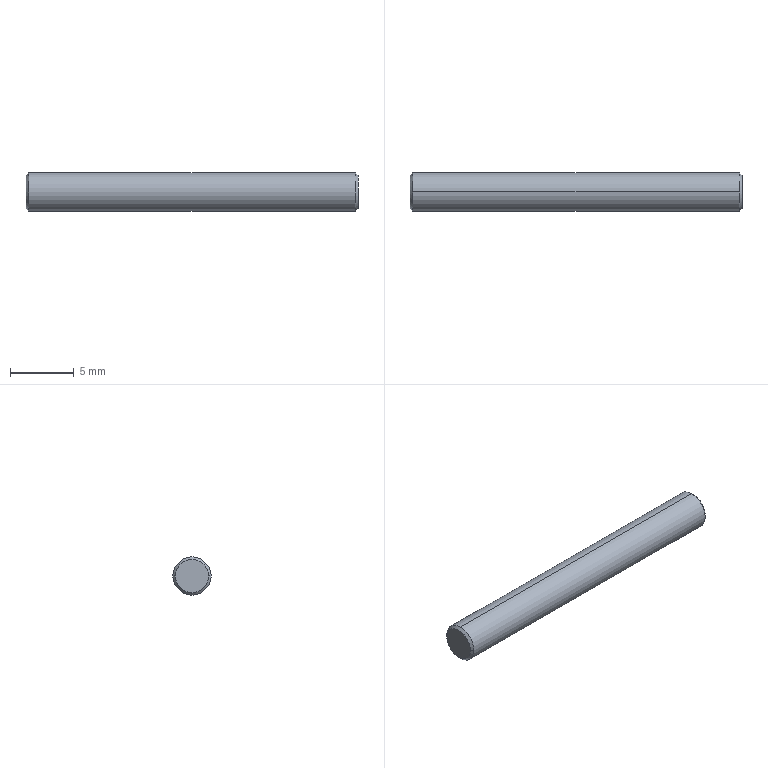Part | STEP file | pin 5_SUS304 | 1 solid | 9 faces | box 26 x 3 x 3 mm | volume 183.423 mm3 | cone 5 | cylinder 2 | plane 2 | commonest cylinder face diameters 3 x2
STEP:
#1=CARTESIAN_POINT('',(0.,0.,0.));
#2=DIRECTION('',(0.,0.,1.));
#3=DIRECTION('',(1.,0.,0.));
#4=AXIS2_PLACEMENT_3D('',#1,#2,#3);
#5=CARTESIAN_POINT('',(12.8,1.5,0.));
#6=VERTEX_POINT('',#5);
#7=CARTESIAN_POINT('',(12.8,0.,-1.5));
#8=VERTEX_POINT('',#7);
#9=CARTESIAN_POINT('',(12.8,0.,0.));
#10=DIRECTION('',(-1.,0.,0.));
#11=DIRECTION('',(0.,0.,1.));
#12=AXIS2_PLACEMENT_3D('',#9,#10,#11);
#13=CIRCLE('',#12,1.5);
#14=CARTESIAN_POINT('',(13.,0.,0.));
#15=DIRECTION('',(-1.,0.,0.));
#16=DIRECTION('',(0.,0.,1.));
#17=AXIS2_PLACEMENT_3D('',#14,#15,#16);
#18=CYLINDRICAL_SURFACE('',#17,1.5);
#19=CARTESIAN_POINT('',(0.,0.2));
#20=DIRECTION('',(1.,0.));
#21=VECTOR('',#20,1.);
#22=LINE('',#19,#21);
#23=(GEOMETRIC_REPRESENTATION_CONTEXT(2)PARAMETRIC_REPRESENTATION_CONTEXT()REPRESENTATION_CONTEXT('',''));
#24=DEFINITIONAL_REPRESENTATION('',(#22),#23);
#25=PCURVE('',#18,#24);
#26=CARTESIAN_POINT('',(12.8,0.,0.));
#27=DIRECTION('',(-1.,0.,0.));
#28=DIRECTION('',(0.,-1.,0.));
#29=AXIS2_PLACEMENT_3D('',#26,#27,#28);
#30=CONICAL_SURFACE('',#29,1.5,0.7854);
#31=CARTESIAN_POINT('',(1.571,0.));
#32=DIRECTION('',(1.,0.));
#33=VECTOR('',#32,1.);
#34=LINE('',#31,#33);
#35=(GEOMETRIC_REPRESENTATION_CONTEXT(2)PARAMETRIC_REPRESENTATION_CONTEXT()REPRESENTATION_CONTEXT('',''));
#36=DEFINITIONAL_REPRESENTATION('',(#34),#35);
#37=PCURVE('',#30,#36);
#38=SURFACE_CURVE('',#13,(#25,#37),.PCURVE_S1.);
#39=EDGE_CURVE('',#6,#8,#38,.T.);
#40=ORIENTED_EDGE('',*,*,#39,.T.);
#41=CARTESIAN_POINT('',(-12.8,0.,-1.5));
#42=VERTEX_POINT('',#41);
#43=CARTESIAN_POINT('',(13.,0.,-1.5));
#44=DIRECTION('',(-1.,0.,0.));
#45=VECTOR('',#44,1.);
#46=LINE('',#43,#45);
#47=CARTESIAN_POINT('',(3.142,0.));
#48=DIRECTION('',(0.,1.));
#49=VECTOR('',#48,1.);
#50=LINE('',#47,#49);
#51=(GEOMETRIC_REPRESENTATION_CONTEXT(2)PARAMETRIC_REPRESENTATION_CONTEXT()REPRESENTATION_CONTEXT('',''));
#52=DEFINITIONAL_REPRESENTATION('',(#50),#51);
#53=PCURVE('',#18,#52);
#54=CARTESIAN_POINT('',(13.,0.,0.));
#55=DIRECTION('',(-1.,0.,0.));
#56=DIRECTION('',(0.,0.,1.));
#57=AXIS2_PLACEMENT_3D('',#54,#55,#56);
#58=CYLINDRICAL_SURFACE('',#57,1.5);
#59=CARTESIAN_POINT('',(3.142,0.));
#60=DIRECTION('',(0.,1.));
#61=VECTOR('',#60,1.);
#62=LINE('',#59,#61);
#63=(GEOMETRIC_REPRESENTATION_CONTEXT(2)PARAMETRIC_REPRESENTATION_CONTEXT()REPRESENTATION_CONTEXT('',''));
#64=DEFINITIONAL_REPRESENTATION('',(#62),#63);
#65=PCURVE('',#58,#64);
#66=SURFACE_CURVE('',#46,(#53,#65),.PCURVE_S1.);
#67=EDGE_CURVE('',#8,#42,#66,.T.);
#68=ORIENTED_EDGE('',*,*,#67,.T.);
#69=CARTESIAN_POINT('',(-12.8,1.5,0.));
#70=VERTEX_POINT('',#69);
#71=CARTESIAN_POINT('',(-12.8,0.,0.));
#72=DIRECTION('',(1.,0.,0.));
#73=DIRECTION('',(0.,0.,1.));
#74=AXIS2_PLACEMENT_3D('',#71,#72,#73);
#75=CIRCLE('',#74,1.5);
#76=CARTESIAN_POINT('',(6.283,25.8));
#77=DIRECTION('',(-1.,0.));
#78=VECTOR('',#77,1.);
#79=LINE('',#76,#78);
#80=(GEOMETRIC_REPRESENTATION_CONTEXT(2)PARAMETRIC_REPRESENTATION_CONTEXT()REPRESENTATION_CONTEXT('',''));
#81=DEFINITIONAL_REPRESENTATION('',(#79),#80);
#82=PCURVE('',#18,#81);
#83=CARTESIAN_POINT('',(-12.8,0.,0.));
#84=DIRECTION('',(1.,0.,0.));
#85=DIRECTION('',(0.,0.,-1.));
#86=AXIS2_PLACEMENT_3D('',#83,#84,#85);
#87=CONICAL_SURFACE('',#86,1.5,0.7854);
#88=CARTESIAN_POINT('',(-3.142,0.));
#89=DIRECTION('',(1.,0.));
#90=VECTOR('',#89,1.);
#91=LINE('',#88,#90);
#92=(GEOMETRIC_REPRESENTATION_CONTEXT(2)PARAMETRIC_REPRESENTATION_CONTEXT()REPRESENTATION_CONTEXT('',''));
#93=DEFINITIONAL_REPRESENTATION('',(#91),#92);
#94=PCURVE('',#87,#93);
#95=SURFACE_CURVE('',#75,(#82,#94),.PCURVE_S1.);
#96=EDGE_CURVE('',#42,#70,#95,.T.);
#97=ORIENTED_EDGE('',*,*,#96,.T.);
#98=CARTESIAN_POINT('',(-12.8,0.,1.5));
#99=VERTEX_POINT('',#98);
#100=CARTESIAN_POINT('',(-12.8,0.,0.));
#101=DIRECTION('',(1.,0.,0.));
#102=DIRECTION('',(0.,0.,1.));
#103=AXIS2_PLACEMENT_3D('',#100,#101,#102);
#104=CIRCLE('',#103,1.5);
#105=CARTESIAN_POINT('',(6.283,25.8));
#106=DIRECTION('',(-1.,0.));
#107=VECTOR('',#106,1.);
#108=LINE('',#105,#107);
#109=(GEOMETRIC_REPRESENTATION_CONTEXT(2)PARAMETRIC_REPRESENTATION_CONTEXT()REPRESENTATION_CONTEXT('',''));
#110=DEFINITIONAL_REPRESENTATION('',(#108),#109);
#111=PCURVE('',#18,#110);
#112=CARTESIAN_POINT('',(-12.8,0.,0.));
#113=DIRECTION('',(1.,0.,0.));
#114=DIRECTION('',(0.,0.,-1.));
#115=AXIS2_PLACEMENT_3D('',#112,#113,#114);
#116=CONICAL_SURFACE('',#115,1.5,0.7854);
#117=CARTESIAN_POINT('',(-3.142,0.));
#118=DIRECTION('',(1.,0.));
#119=VECTOR('',#118,1.);
#120=LINE('',#117,#119);
#121=(GEOMETRIC_REPRESENTATION_CONTEXT(2)PARAMETRIC_REPRESENTATION_CONTEXT()REPRESENTATION_CONTEXT('',''));
#122=DEFINITIONAL_REPRESENTATION('',(#120),#121);
#123=PCURVE('',#116,#122);
#124=SURFACE_CURVE('',#104,(#111,#123),.PCURVE_S1.);
#125=EDGE_CURVE('',#70,#99,#124,.T.);
#126=ORIENTED_EDGE('',*,*,#125,.T.);
#127=CARTESIAN_POINT('',(12.8,0.,1.5));
#128=VERTEX_POINT('',#127);
#129=CARTESIAN_POINT('',(13.,0.,1.5));
#130=DIRECTION('',(-1.,0.,0.));
#131=VECTOR('',#130,1.);
#132=LINE('',#129,#131);
#133=CARTESIAN_POINT('',(0.,0.));
#134=DIRECTION('',(0.,1.));
#135=VECTOR('',#134,1.);
#136=LINE('',#133,#135);
#137=(GEOMETRIC_REPRESENTATION_CONTEXT(2)PARAMETRIC_REPRESENTATION_CONTEXT()REPRESENTATION_CONTEXT('',''));
#138=DEFINITIONAL_REPRESENTATION('',(#136),#137);
#139=PCURVE('',#18,#138);
#140=CARTESIAN_POINT('',(6.283,0.));
#141=DIRECTION('',(0.,1.));
#142=VECTOR('',#141,1.);
#143=LINE('',#140,#142);
#144=(GEOMETRIC_REPRESENTATION_CONTEXT(2)PARAMETRIC_REPRESENTATION_CONTEXT()REPRESENTATION_CONTEXT('',''));
#145=DEFINITIONAL_REPRESENTATION('',(#143),#144);
#146=PCURVE('',#58,#145);
#147=SURFACE_CURVE('',#132,(#139,#146),.PCURVE_S1.);
#148=EDGE_CURVE('',#128,#99,#147,.T.);
#149=ORIENTED_EDGE('',*,*,#148,.F.);
#150=CARTESIAN_POINT('',(12.8,0.,0.));
#151=DIRECTION('',(-1.,0.,0.));
#152=DIRECTION('',(0.,0.,1.));
#153=AXIS2_PLACEMENT_3D('',#150,#151,#152);
#154=CIRCLE('',#153,1.5);
#155=CARTESIAN_POINT('',(0.,0.2));
#156=DIRECTION('',(1.,0.));
#157=VECTOR('',#156,1.);
#158=LINE('',#155,#157);
#159=(GEOMETRIC_REPRESENTATION_CONTEXT(2)PARAMETRIC_REPRESENTATION_CONTEXT()REPRESENTATION_CONTEXT('',''));
#160=DEFINITIONAL_REPRESENTATION('',(#158),#159);
#161=PCURVE('',#18,#160);
#162=CARTESIAN_POINT('',(12.8,0.,0.));
#163=DIRECTION('',(-1.,0.,0.));
#164=DIRECTION('',(0.,-1.,0.));
#165=AXIS2_PLACEMENT_3D('',#162,#163,#164);
#166=CONICAL_SURFACE('',#165,1.5,0.7854);
#167=CARTESIAN_POINT('',(1.571,0.));
#168=DIRECTION('',(1.,0.));
#169=VECTOR('',#168,1.);
#170=LINE('',#167,#169);
#171=(GEOMETRIC_REPRESENTATION_CONTEXT(2)PARAMETRIC_REPRESENTATION_CONTEXT()REPRESENTATION_CONTEXT('',''));
#172=DEFINITIONAL_REPRESENTATION('',(#170),#171);
#173=PCURVE('',#166,#172);
#174=SURFACE_CURVE('',#154,(#161,#173),.PCURVE_S1.);
#175=EDGE_CURVE('',#128,#6,#174,.T.);
#176=ORIENTED_EDGE('',*,*,#175,.T.);
#177=EDGE_LOOP('',(#40,#68,#97,#126,#149,#176));
#178=FACE_BOUND('',#177,.T.);
#179=ADVANCED_FACE('',(#178),#18,.T.);
#180=CARTESIAN_POINT('',(13.,-1.3,0.));
#181=VERTEX_POINT('',#180);
#182=CARTESIAN_POINT('',(13.,1.3,0.));
#183=VERTEX_POINT('',#182);
#184=CARTESIAN_POINT('',(13.,0.,0.));
#185=DIRECTION('',(-1.,0.,0.));
#186=DIRECTION('',(0.,-1.,0.));
#187=AXIS2_PLACEMENT_3D('',#184,#185,#186);
#188=CIRCLE('',#187,1.3);
#189=CARTESIAN_POINT('',(0.,-0.2));
#190=DIRECTION('',(1.,0.));
#191=VECTOR('',#190,1.);
#192=LINE('',#189,#191);
#193=(GEOMETRIC_REPRESENTATION_CONTEXT(2)PARAMETRIC_REPRESENTATION_CONTEXT()REPRESENTATION_CONTEXT('',''));
#194=DEFINITIONAL_REPRESENTATION('',(#192),#193);
#195=PCURVE('',#166,#194);
#196=CARTESIAN_POINT('',(13.,0.,0.));
#197=DIRECTION('',(1.,0.,0.));
#198=DIRECTION('',(0.,0.,-1.));
#199=AXIS2_PLACEMENT_3D('',#196,#197,#198);
#200=PLANE('',#199);
#201=CARTESIAN_POINT('',(0.,-1.3));
#202=CARTESIAN_POINT('',(-2.252,-1.3));
#203=CARTESIAN_POINT('',(-1.126,0.65));
#204=CARTESIAN_POINT('',(0.,2.6));
#205=CARTESIAN_POINT('',(1.126,0.65));
#206=CARTESIAN_POINT('',(2.252,-1.3));
#207=CARTESIAN_POINT('',(0.,-1.3));
#208=(BOUNDED_CURVE()B_SPLINE_CURVE(2,(#201,#202,#203,#204,#205,#206,#207),.UNSPECIFIED.,.T.,.F.)B_SPLINE_CURVE_WITH_KNOTS((1,2,2,2,2,1),(-2.094,0.,2.094,4.189,6.283,8.378),.UNSPECIFIED.)CURVE()GEOMETRIC_REPRESENTATION_ITEM()RATIONAL_B_SPLINE_CURVE((1.,0.5,1.,0.5,1.,0.5,1.))REPRESENTATION_ITEM(''));
#209=(GEOMETRIC_REPRESENTATION_CONTEXT(2)PARAMETRIC_REPRESENTATION_CONTEXT()REPRESENTATION_CONTEXT('',''));
#210=DEFINITIONAL_REPRESENTATION('',(#208),#209);
#211=PCURVE('',#200,#210);
#212=SURFACE_CURVE('',#188,(#195,#211),.PCURVE_S1.);
#213=EDGE_CURVE('',#181,#183,#212,.T.);
#214=ORIENTED_EDGE('',*,*,#213,.T.);
#215=CARTESIAN_POINT('',(12.8,1.5,0.));
#216=DIRECTION('',(-0.7071,0.7071,0.));
#217=VECTOR('',#216,1.);
#218=LINE('',#215,#217);
#219=CARTESIAN_POINT('',(3.142,0.));
#220=DIRECTION('',(0.,1.));
#221=VECTOR('',#220,1.);
#222=LINE('',#219,#221);
#223=(GEOMETRIC_REPRESENTATION_CONTEXT(2)PARAMETRIC_REPRESENTATION_CONTEXT()REPRESENTATION_CONTEXT('',''));
#224=DEFINITIONAL_REPRESENTATION('',(#222),#223);
#225=PCURVE('',#166,#224);
#226=CARTESIAN_POINT('',(3.142,0.));
#227=DIRECTION('',(0.,1.));
#228=VECTOR('',#227,1.);
#229=LINE('',#226,#228);
#230=(GEOMETRIC_REPRESENTATION_CONTEXT(2)PARAMETRIC_REPRESENTATION_CONTEXT()REPRESENTATION_CONTEXT('',''));
#231=DEFINITIONAL_REPRESENTATION('',(#229),#230);
#232=PCURVE('',#30,#231);
#233=SURFACE_CURVE('',#218,(#225,#232),.PCURVE_S1.);
#234=EDGE_CURVE('',#183,#6,#233,.T.);
#235=ORIENTED_EDGE('',*,*,#234,.T.);
#236=ORIENTED_EDGE('',*,*,#175,.F.);
#237=CARTESIAN_POINT('',(12.8,-1.5,0.));
#238=VERTEX_POINT('',#237);
#239=CARTESIAN_POINT('',(12.8,0.,0.));
#240=DIRECTION('',(-1.,0.,0.));
#241=DIRECTION('',(0.,0.,1.));
#242=AXIS2_PLACEMENT_3D('',#239,#240,#241);
#243=CIRCLE('',#242,1.5);
#244=CARTESIAN_POINT('',(-4.712,0.));
#245=DIRECTION('',(1.,0.));
#246=VECTOR('',#245,1.);
#247=LINE('',#244,#246);
#248=(GEOMETRIC_REPRESENTATION_CONTEXT(2)PARAMETRIC_REPRESENTATION_CONTEXT()REPRESENTATION_CONTEXT('',''));
#249=DEFINITIONAL_REPRESENTATION('',(#247),#248);
#250=PCURVE('',#166,#249);
#251=CARTESIAN_POINT('',(0.,0.2));
#252=DIRECTION('',(1.,0.));
#253=VECTOR('',#252,1.);
#254=LINE('',#251,#253);
#255=(GEOMETRIC_REPRESENTATION_CONTEXT(2)PARAMETRIC_REPRESENTATION_CONTEXT()REPRESENTATION_CONTEXT('',''));
#256=DEFINITIONAL_REPRESENTATION('',(#254),#255);
#257=PCURVE('',#58,#256);
#258=SURFACE_CURVE('',#243,(#250,#257),.PCURVE_S1.);
#259=EDGE_CURVE('',#238,#128,#258,.T.);
#260=ORIENTED_EDGE('',*,*,#259,.F.);
#261=CARTESIAN_POINT('',(12.8,-1.5,0.));
#262=DIRECTION('',(-0.7071,-0.7071,0.));
#263=VECTOR('',#262,1.);
#264=LINE('',#261,#263);
#265=CARTESIAN_POINT('',(0.,0.));
#266=DIRECTION('',(0.,1.));
#267=VECTOR('',#266,1.);
#268=LINE('',#265,#267);
#269=(GEOMETRIC_REPRESENTATION_CONTEXT(2)PARAMETRIC_REPRESENTATION_CONTEXT()REPRESENTATION_CONTEXT('',''));
#270=DEFINITIONAL_REPRESENTATION('',(#268),#269);
#271=PCURVE('',#166,#270);
#272=CARTESIAN_POINT('',(6.283,0.));
#273=DIRECTION('',(0.,1.));
#274=VECTOR('',#273,1.);
#275=LINE('',#272,#274);
#276=(GEOMETRIC_REPRESENTATION_CONTEXT(2)PARAMETRIC_REPRESENTATION_CONTEXT()REPRESENTATION_CONTEXT('',''));
#277=DEFINITIONAL_REPRESENTATION('',(#275),#276);
#278=PCURVE('',#30,#277);
#279=SURFACE_CURVE('',#264,(#271,#278),.PCURVE_S1.);
#280=EDGE_CURVE('',#181,#238,#279,.T.);
#281=ORIENTED_EDGE('',*,*,#280,.F.);
#282=EDGE_LOOP('',(#214,#235,#236,#260,#281));
#283=FACE_BOUND('',#282,.T.);
#284=ADVANCED_FACE('',(#283),#166,.T.);
#285=CARTESIAN_POINT('',(-13.,-1.3,0.));
#286=VERTEX_POINT('',#285);
#287=CARTESIAN_POINT('',(-13.,0.,-1.3));
#288=VERTEX_POINT('',#287);
#289=CARTESIAN_POINT('',(-13.,0.,0.));
#290=DIRECTION('',(1.,0.,0.));
#291=DIRECTION('',(0.,0.,-1.));
#292=AXIS2_PLACEMENT_3D('',#289,#290,#291);
#293=CIRCLE('',#292,1.3);
#294=CARTESIAN_POINT('',(-12.8,0.,0.));
#295=DIRECTION('',(1.,0.,0.));
#296=DIRECTION('',(0.,0.,-1.));
#297=AXIS2_PLACEMENT_3D('',#294,#295,#296);
#298=CONICAL_SURFACE('',#297,1.5,0.7854);
#299=CARTESIAN_POINT('',(0.,-0.2));
#300=DIRECTION('',(1.,0.));
#301=VECTOR('',#300,1.);
#302=LINE('',#299,#301);
#303=(GEOMETRIC_REPRESENTATION_CONTEXT(2)PARAMETRIC_REPRESENTATION_CONTEXT()REPRESENTATION_CONTEXT('',''));
#304=DEFINITIONAL_REPRESENTATION('',(#302),#303);
#305=PCURVE('',#298,#304);
#306=CARTESIAN_POINT('',(-13.,0.,0.));
#307=DIRECTION('',(1.,0.,0.));
#308=DIRECTION('',(0.,0.,-1.));
#309=AXIS2_PLACEMENT_3D('',#306,#307,#308);
#310=PLANE('',#309);
#311=CARTESIAN_POINT('',(0.,0.));
#312=DIRECTION('',(1.,0.));
#313=AXIS2_PLACEMENT_2D('',#311,#312);
#314=CIRCLE('',#313,1.3);
#315=(GEOMETRIC_REPRESENTATION_CONTEXT(2)PARAMETRIC_REPRESENTATION_CONTEXT()REPRESENTATION_CONTEXT('',''));
#316=DEFINITIONAL_REPRESENTATION('',(#314),#315);
#317=PCURVE('',#310,#316);
#318=SURFACE_CURVE('',#293,(#305,#317),.PCURVE_S1.);
#319=EDGE_CURVE('',#286,#288,#318,.T.);
#320=ORIENTED_EDGE('',*,*,#319,.T.);
#321=CARTESIAN_POINT('',(-12.8,0.,-1.5));
#322=DIRECTION('',(0.7071,0.,-0.7071));
#323=VECTOR('',#322,1.);
#324=LINE('',#321,#323);
#325=CARTESIAN_POINT('',(6.283,0.));
#326=DIRECTION('',(0.,1.));
#327=VECTOR('',#326,1.);
#328=LINE('',#325,#327);
#329=(GEOMETRIC_REPRESENTATION_CONTEXT(2)PARAMETRIC_REPRESENTATION_CONTEXT()REPRESENTATION_CONTEXT('',''));
#330=DEFINITIONAL_REPRESENTATION('',(#328),#329);
#331=PCURVE('',#298,#330);
#332=CARTESIAN_POINT('',(0.,0.));
#333=DIRECTION('',(0.,1.));
#334=VECTOR('',#333,1.);
#335=LINE('',#332,#334);
#336=(GEOMETRIC_REPRESENTATION_CONTEXT(2)PARAMETRIC_REPRESENTATION_CONTEXT()REPRESENTATION_CONTEXT('',''));
#337=DEFINITIONAL_REPRESENTATION('',(#335),#336);
#338=PCURVE('',#87,#337);
#339=SURFACE_CURVE('',#324,(#331,#338),.PCURVE_S1.);
#340=EDGE_CURVE('',#288,#42,#339,.T.);
#341=ORIENTED_EDGE('',*,*,#340,.T.);
#342=CARTESIAN_POINT('',(-12.8,-1.5,0.));
#343=VERTEX_POINT('',#342);
#344=CARTESIAN_POINT('',(-12.8,0.,0.));
#345=DIRECTION('',(1.,0.,0.));
#346=DIRECTION('',(0.,0.,1.));
#347=AXIS2_PLACEMENT_3D('',#344,#345,#346);
#348=CIRCLE('',#347,1.5);
#349=CARTESIAN_POINT('',(3.142,0.));
#350=DIRECTION('',(1.,0.));
#351=VECTOR('',#350,1.);
#352=LINE('',#349,#351);
#353=(GEOMETRIC_REPRESENTATION_CONTEXT(2)PARAMETRIC_REPRESENTATION_CONTEXT()REPRESENTATION_CONTEXT('',''));
#354=DEFINITIONAL_REPRESENTATION('',(#352),#353);
#355=PCURVE('',#298,#354);
#356=CARTESIAN_POINT('',(6.283,25.8));
#357=DIRECTION('',(-1.,0.));
#358=VECTOR('',#357,1.);
#359=LINE('',#356,#358);
#360=(GEOMETRIC_REPRESENTATION_CONTEXT(2)PARAMETRIC_REPRESENTATION_CONTEXT()REPRESENTATION_CONTEXT('',''));
#361=DEFINITIONAL_REPRESENTATION('',(#359),#360);
#362=PCURVE('',#58,#361);
#363=SURFACE_CURVE('',#348,(#355,#362),.PCURVE_S1.);
#364=EDGE_CURVE('',#343,#42,#363,.T.);
#365=ORIENTED_EDGE('',*,*,#364,.F.);
#366=CARTESIAN_POINT('',(498985.7,-499000.,0.));
#367=DIRECTION('',(0.7071,-0.7071,0.));
#368=VECTOR('',#367,1.);
#369=LINE('',#366,#368);
#370=CARTESIAN_POINT('',(4.712,498998.5));
#371=DIRECTION('',(0.,1.));
#372=VECTOR('',#371,1.);
#373=LINE('',#370,#372);
#374=(GEOMETRIC_REPRESENTATION_CONTEXT(2)PARAMETRIC_REPRESENTATION_CONTEXT()REPRESENTATION_CONTEXT('',''));
#375=DEFINITIONAL_REPRESENTATION('',(#373),#374);
#376=PCURVE('',#298,#375);
#377=CARTESIAN_POINT('',(4.712,498998.5));
#378=DIRECTION('',(0.,1.));
#379=VECTOR('',#378,1.);
#380=LINE('',#377,#379);
#381=(GEOMETRIC_REPRESENTATION_CONTEXT(2)PARAMETRIC_REPRESENTATION_CONTEXT()REPRESENTATION_CONTEXT('',''));
#382=DEFINITIONAL_REPRESENTATION('',(#380),#381);
#383=PCURVE('',#116,#382);
#384=SURFACE_CURVE('',#369,(#376,#383),.PCURVE_S1.);
#385=EDGE_CURVE('',#286,#343,#384,.T.);
#386=ORIENTED_EDGE('',*,*,#385,.F.);
#387=EDGE_LOOP('',(#320,#341,#365,#386));
#388=FACE_BOUND('',#387,.T.);
#389=ADVANCED_FACE('',(#388),#298,.T.);
#390=ORIENTED_EDGE('',*,*,#67,.F.);
#391=CARTESIAN_POINT('',(12.8,0.,0.));
#392=DIRECTION('',(-1.,0.,0.));
#393=DIRECTION('',(0.,0.,1.));
#394=AXIS2_PLACEMENT_3D('',#391,#392,#393);
#395=CIRCLE('',#394,1.5);
#396=CARTESIAN_POINT('',(0.,0.2));
#397=DIRECTION('',(1.,0.));
#398=VECTOR('',#397,1.);
#399=LINE('',#396,#398);
#400=(GEOMETRIC_REPRESENTATION_CONTEXT(2)PARAMETRIC_REPRESENTATION_CONTEXT()REPRESENTATION_CONTEXT('',''));
#401=DEFINITIONAL_REPRESENTATION('',(#399),#400);
#402=PCURVE('',#58,#401);
#403=CARTESIAN_POINT('',(1.571,0.));
#404=DIRECTION('',(1.,0.));
#405=VECTOR('',#404,1.);
#406=LINE('',#403,#405);
#407=(GEOMETRIC_REPRESENTATION_CONTEXT(2)PARAMETRIC_REPRESENTATION_CONTEXT()REPRESENTATION_CONTEXT('',''));
#408=DEFINITIONAL_REPRESENTATION('',(#406),#407);
#409=PCURVE('',#30,#408);
#410=SURFACE_CURVE('',#395,(#402,#409),.PCURVE_S1.);
#411=EDGE_CURVE('',#8,#238,#410,.T.);
#412=ORIENTED_EDGE('',*,*,#411,.T.);
#413=ORIENTED_EDGE('',*,*,#259,.T.);
#414=ORIENTED_EDGE('',*,*,#148,.T.);
#415=CARTESIAN_POINT('',(-12.8,0.,0.));
#416=DIRECTION('',(1.,0.,0.));
#417=DIRECTION('',(0.,0.,1.));
#418=AXIS2_PLACEMENT_3D('',#415,#416,#417);
#419=CIRCLE('',#418,1.5);
#420=CARTESIAN_POINT('',(6.283,25.8));
#421=DIRECTION('',(-1.,0.));
#422=VECTOR('',#421,1.);
#423=LINE('',#420,#422);
#424=(GEOMETRIC_REPRESENTATION_CONTEXT(2)PARAMETRIC_REPRESENTATION_CONTEXT()REPRESENTATION_CONTEXT('',''));
#425=DEFINITIONAL_REPRESENTATION('',(#423),#424);
#426=PCURVE('',#58,#425);
#427=CARTESIAN_POINT('',(3.142,0.));
#428=DIRECTION('',(1.,0.));
#429=VECTOR('',#428,1.);
#430=LINE('',#427,#429);
#431=(GEOMETRIC_REPRESENTATION_CONTEXT(2)PARAMETRIC_REPRESENTATION_CONTEXT()REPRESENTATION_CONTEXT('',''));
#432=DEFINITIONAL_REPRESENTATION('',(#430),#431);
#433=PCURVE('',#116,#432);
#434=SURFACE_CURVE('',#419,(#426,#433),.PCURVE_S1.);
#435=EDGE_CURVE('',#99,#343,#434,.T.);
#436=ORIENTED_EDGE('',*,*,#435,.T.);
#437=ORIENTED_EDGE('',*,*,#364,.T.);
#438=EDGE_LOOP('',(#390,#412,#413,#414,#436,#437));
#439=FACE_BOUND('',#438,.T.);
#440=ADVANCED_FACE('',(#439),#58,.T.);
#441=ORIENTED_EDGE('',*,*,#234,.F.);
#442=CARTESIAN_POINT('',(13.,0.,0.));
#443=DIRECTION('',(-1.,0.,0.));
#444=DIRECTION('',(0.,-1.,0.));
#445=AXIS2_PLACEMENT_3D('',#442,#443,#444);
#446=CIRCLE('',#445,1.3);
#447=CARTESIAN_POINT('',(0.,-0.2));
#448=DIRECTION('',(1.,0.));
#449=VECTOR('',#448,1.);
#450=LINE('',#447,#449);
#451=(GEOMETRIC_REPRESENTATION_CONTEXT(2)PARAMETRIC_REPRESENTATION_CONTEXT()REPRESENTATION_CONTEXT('',''));
#452=DEFINITIONAL_REPRESENTATION('',(#450),#451);
#453=PCURVE('',#30,#452);
#454=CARTESIAN_POINT('',(0.,-1.3));
#455=CARTESIAN_POINT('',(-2.252,-1.3));
#456=CARTESIAN_POINT('',(-1.126,0.65));
#457=CARTESIAN_POINT('',(0.,2.6));
#458=CARTESIAN_POINT('',(1.126,0.65));
#459=CARTESIAN_POINT('',(2.252,-1.3));
#460=CARTESIAN_POINT('',(0.,-1.3));
#461=(BOUNDED_CURVE()B_SPLINE_CURVE(2,(#454,#455,#456,#457,#458,#459,#460),.UNSPECIFIED.,.T.,.F.)B_SPLINE_CURVE_WITH_KNOTS((1,2,2,2,2,1),(-2.094,0.,2.094,4.189,6.283,8.378),.UNSPECIFIED.)CURVE()GEOMETRIC_REPRESENTATION_ITEM()RATIONAL_B_SPLINE_CURVE((1.,0.5,1.,0.5,1.,0.5,1.))REPRESENTATION_ITEM(''));
#462=(GEOMETRIC_REPRESENTATION_CONTEXT(2)PARAMETRIC_REPRESENTATION_CONTEXT()REPRESENTATION_CONTEXT('',''));
#463=DEFINITIONAL_REPRESENTATION('',(#461),#462);
#464=PCURVE('',#200,#463);
#465=SURFACE_CURVE('',#446,(#453,#464),.PCURVE_S1.);
#466=EDGE_CURVE('',#183,#181,#465,.T.);
#467=ORIENTED_EDGE('',*,*,#466,.T.);
#468=ORIENTED_EDGE('',*,*,#280,.T.);
#469=ORIENTED_EDGE('',*,*,#411,.F.);
#470=ORIENTED_EDGE('',*,*,#39,.F.);
#471=EDGE_LOOP('',(#441,#467,#468,#469,#470));
#472=FACE_BOUND('',#471,.T.);
#473=ADVANCED_FACE('',(#472),#30,.T.);
#474=ORIENTED_EDGE('',*,*,#125,.F.);
#475=CARTESIAN_POINT('',(-13.,1.3,0.));
#476=VERTEX_POINT('',#475);
#477=CARTESIAN_POINT('',(498985.7,499000.,0.));
#478=DIRECTION('',(-0.7071,-0.7071,0.));
#479=VECTOR('',#478,1.);
#480=LINE('',#477,#479);
#481=CARTESIAN_POINT('',(1.571,498998.5));
#482=DIRECTION('',(0.,-1.));
#483=VECTOR('',#482,1.);
#484=LINE('',#481,#483);
#485=(GEOMETRIC_REPRESENTATION_CONTEXT(2)PARAMETRIC_REPRESENTATION_CONTEXT()REPRESENTATION_CONTEXT('',''));
#486=DEFINITIONAL_REPRESENTATION('',(#484),#485);
#487=PCURVE('',#116,#486);
#488=CARTESIAN_POINT('',(1.571,498998.5));
#489=DIRECTION('',(0.,-1.));
#490=VECTOR('',#489,1.);
#491=LINE('',#488,#490);
#492=(GEOMETRIC_REPRESENTATION_CONTEXT(2)PARAMETRIC_REPRESENTATION_CONTEXT()REPRESENTATION_CONTEXT('',''));
#493=DEFINITIONAL_REPRESENTATION('',(#491),#492);
#494=PCURVE('',#87,#493);
#495=SURFACE_CURVE('',#480,(#487,#494),.PCURVE_S1.);
#496=EDGE_CURVE('',#70,#476,#495,.T.);
#497=ORIENTED_EDGE('',*,*,#496,.T.);
#498=CARTESIAN_POINT('',(-13.,0.,0.));
#499=DIRECTION('',(1.,0.,0.));
#500=DIRECTION('',(0.,0.,-1.));
#501=AXIS2_PLACEMENT_3D('',#498,#499,#500);
#502=CIRCLE('',#501,1.3);
#503=CARTESIAN_POINT('',(0.,-0.2));
#504=DIRECTION('',(1.,0.));
#505=VECTOR('',#504,1.);
#506=LINE('',#503,#505);
#507=(GEOMETRIC_REPRESENTATION_CONTEXT(2)PARAMETRIC_REPRESENTATION_CONTEXT()REPRESENTATION_CONTEXT('',''));
#508=DEFINITIONAL_REPRESENTATION('',(#506),#507);
#509=PCURVE('',#116,#508);
#510=CARTESIAN_POINT('',(0.,0.));
#511=DIRECTION('',(1.,0.));
#512=AXIS2_PLACEMENT_2D('',#510,#511);
#513=CIRCLE('',#512,1.3);
#514=(GEOMETRIC_REPRESENTATION_CONTEXT(2)PARAMETRIC_REPRESENTATION_CONTEXT()REPRESENTATION_CONTEXT('',''));
#515=DEFINITIONAL_REPRESENTATION('',(#513),#514);
#516=PCURVE('',#310,#515);
#517=SURFACE_CURVE('',#502,(#509,#516),.PCURVE_S1.);
#518=EDGE_CURVE('',#476,#286,#517,.T.);
#519=ORIENTED_EDGE('',*,*,#518,.T.);
#520=ORIENTED_EDGE('',*,*,#385,.T.);
#521=ORIENTED_EDGE('',*,*,#435,.F.);
#522=EDGE_LOOP('',(#474,#497,#519,#520,#521));
#523=FACE_BOUND('',#522,.T.);
#524=ADVANCED_FACE('',(#523),#116,.T.);
#525=ORIENTED_EDGE('',*,*,#340,.F.);
#526=CARTESIAN_POINT('',(-13.,0.,0.));
#527=DIRECTION('',(1.,0.,0.));
#528=DIRECTION('',(0.,0.,-1.));
#529=AXIS2_PLACEMENT_3D('',#526,#527,#528);
#530=CIRCLE('',#529,1.3);
#531=CARTESIAN_POINT('',(0.,-0.2));
#532=DIRECTION('',(1.,0.));
#533=VECTOR('',#532,1.);
#534=LINE('',#531,#533);
#535=(GEOMETRIC_REPRESENTATION_CONTEXT(2)PARAMETRIC_REPRESENTATION_CONTEXT()REPRESENTATION_CONTEXT('',''));
#536=DEFINITIONAL_REPRESENTATION('',(#534),#535);
#537=PCURVE('',#87,#536);
#538=CARTESIAN_POINT('',(0.,0.));
#539=DIRECTION('',(1.,0.));
#540=AXIS2_PLACEMENT_2D('',#538,#539);
#541=CIRCLE('',#540,1.3);
#542=(GEOMETRIC_REPRESENTATION_CONTEXT(2)PARAMETRIC_REPRESENTATION_CONTEXT()REPRESENTATION_CONTEXT('',''));
#543=DEFINITIONAL_REPRESENTATION('',(#541),#542);
#544=PCURVE('',#310,#543);
#545=SURFACE_CURVE('',#530,(#537,#544),.PCURVE_S1.);
#546=EDGE_CURVE('',#288,#476,#545,.T.);
#547=ORIENTED_EDGE('',*,*,#546,.T.);
#548=ORIENTED_EDGE('',*,*,#496,.F.);
#549=ORIENTED_EDGE('',*,*,#96,.F.);
#550=EDGE_LOOP('',(#525,#547,#548,#549));
#551=FACE_BOUND('',#550,.T.);
#552=ADVANCED_FACE('',(#551),#87,.T.);
#553=ORIENTED_EDGE('',*,*,#213,.F.);
#554=ORIENTED_EDGE('',*,*,#466,.F.);
#555=EDGE_LOOP('',(#553,#554));
#556=FACE_BOUND('',#555,.T.);
#557=ADVANCED_FACE('',(#556),#200,.T.);
#558=ORIENTED_EDGE('',*,*,#319,.F.);
#559=ORIENTED_EDGE('',*,*,#518,.F.);
#560=ORIENTED_EDGE('',*,*,#546,.F.);
#561=EDGE_LOOP('',(#558,#559,#560));
#562=FACE_BOUND('',#561,.T.);
#563=ADVANCED_FACE('',(#562),#310,.F.);
#564=CLOSED_SHELL('',(#179,#284,#389,#440,#473,#524,#552,#557,#563));
#565=MANIFOLD_SOLID_BREP('',#564);
#566=(LENGTH_UNIT()NAMED_UNIT(*)SI_UNIT(.MILLI.,.METRE.));
#567=UNCERTAINTY_MEASURE_WITH_UNIT(LENGTH_MEASURE(0.0000001),#566,'','');
#568=(NAMED_UNIT(*)PLANE_ANGLE_UNIT()SI_UNIT($,.RADIAN.));
#569=(NAMED_UNIT(*)SI_UNIT($,.STERADIAN.)SOLID_ANGLE_UNIT());
#570=(GEOMETRIC_REPRESENTATION_CONTEXT(3)GLOBAL_UNCERTAINTY_ASSIGNED_CONTEXT((#567))GLOBAL_UNIT_ASSIGNED_CONTEXT((#566,#568,#569))REPRESENTATION_CONTEXT('',''));
#571=ADVANCED_BREP_SHAPE_REPRESENTATION('',(#4,#565),#570);